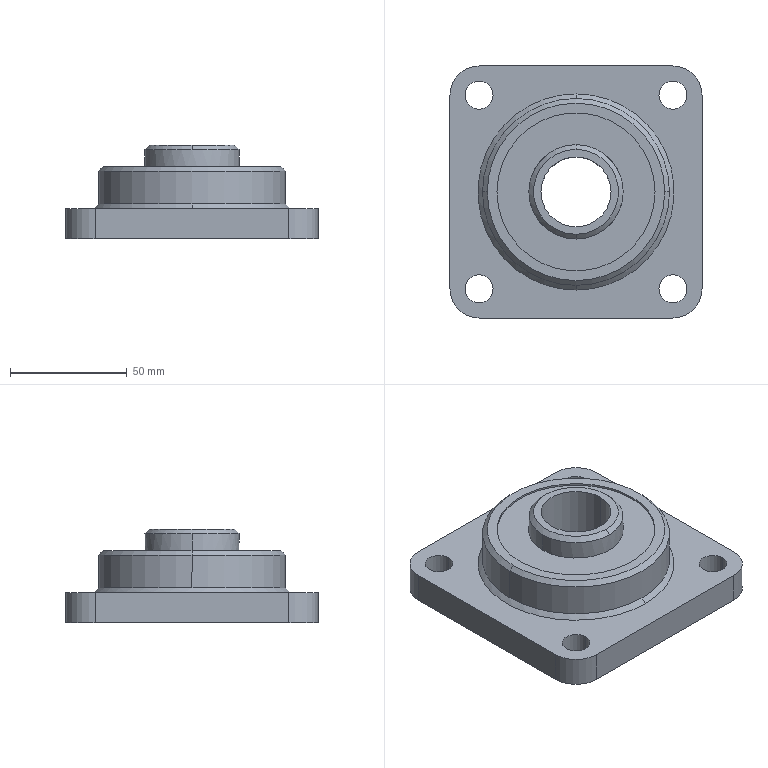Part | STEP file | UCF206_1 | 1 solid | 35 faces | box 108 x 108 x 40.2 mm | volume 215781 mm3 | cylinder 20 | plane 9 | cone 6 | commonest cylinder face diameters 12 x8 25 x4 30 x2 40.4 x2 67.69 x2 80 x2